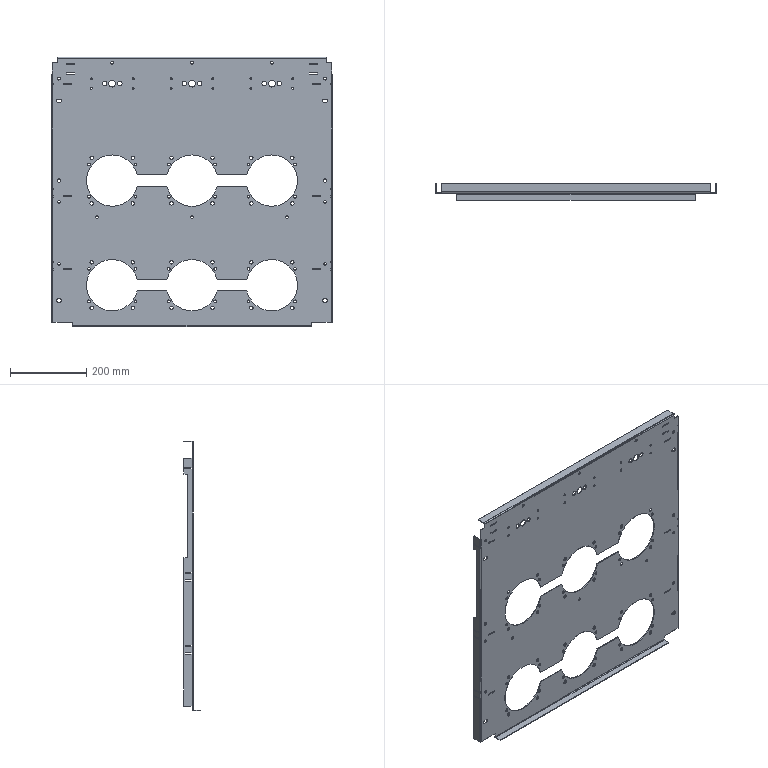Part | STEP file | 1 solid | 406 faces | box 739 x 43 x 710 mm | volume 942644 mm3 | cylinder 220 | plane 186 | commonest cylinder face diameters 7 x86 9 x60 5.2 x24 135 x18 3 x14 12 x12